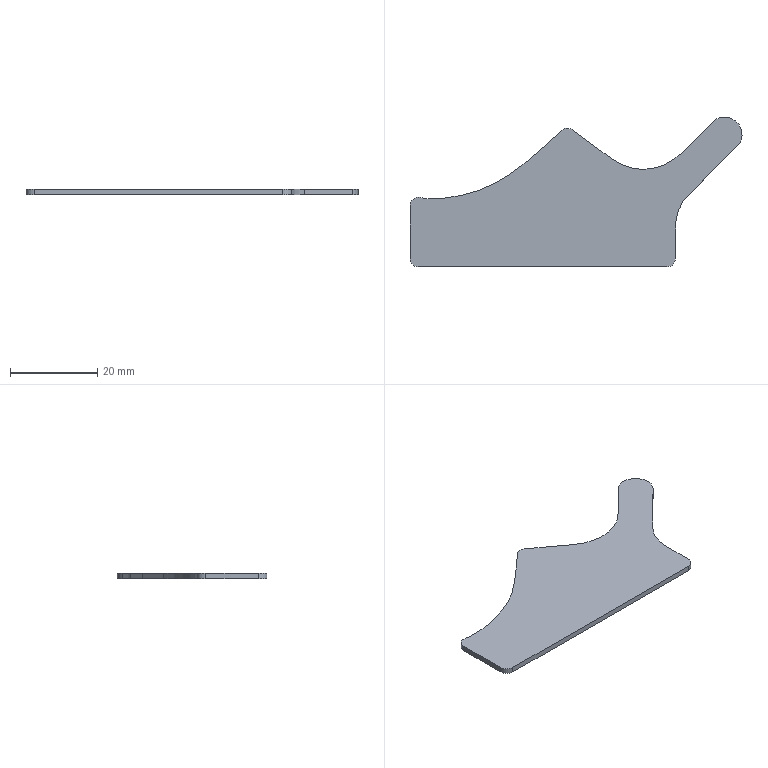Part | STEP file | gslz 2016.10.28-13_id158_x_t | 1 solid | 19 faces | box 76.112 x 34.355 x 1.25 mm | volume 1903 mm3 | plane 10 | cylinder 9 | commonest cylinder face diameters 4 x5 8 x1 20 x1 24 x1 66 x1